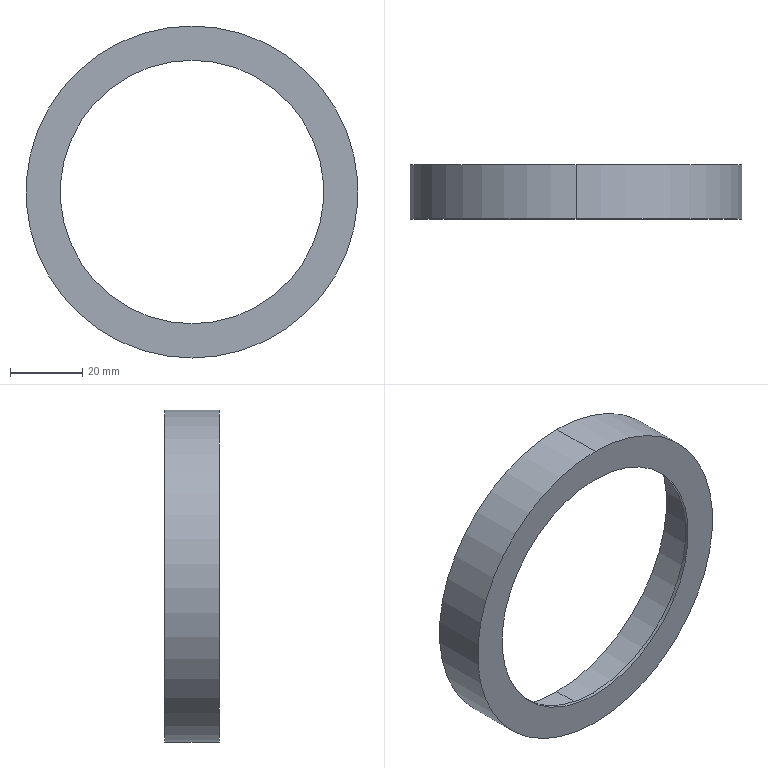Part | SolidWorks | features Revolution 1 | 1 solid | 9 faces | box 92 x 15 x 92 mm | volume 14205 mm3 | cylinder 6 | plane 3 | commonest cylinder face diameters 73 x2 86 x2 92 x2
STEP:
#1=CARTESIAN_POINT('',(0.,15.,43.));
#2=VERTEX_POINT('',#1);
#3=CARTESIAN_POINT('',(0.,15.,-43.));
#4=VERTEX_POINT('',#3);
#5=CARTESIAN_POINT('',(0.,15.,0.));
#6=DIRECTION('',(0.,-1.,0.));
#7=DIRECTION('',(0.,0.,-1.));
#8=AXIS2_PLACEMENT_3D('',#5,#6,#7);
#9=CIRCLE('',#8,43.);
#10=EDGE_CURVE('',#2,#4,#9,.T.);
#11=ORIENTED_EDGE('',*,*,#10,.F.);
#12=CARTESIAN_POINT('',(0.,1.,43.));
#13=VERTEX_POINT('',#12);
#14=CARTESIAN_POINT('',(0.,0.,43.));
#15=DIRECTION('',(0.,-1.,0.));
#16=VECTOR('',#15,1000.);
#17=LINE('',#14,#16);
#18=EDGE_CURVE('',#2,#13,#17,.T.);
#19=ORIENTED_EDGE('',*,*,#18,.T.);
#20=CARTESIAN_POINT('',(0.,1.,-43.));
#21=VERTEX_POINT('',#20);
#22=CARTESIAN_POINT('',(0.,1.,0.));
#23=DIRECTION('',(0.,-1.,0.));
#24=DIRECTION('',(0.,0.,-1.));
#25=AXIS2_PLACEMENT_3D('',#22,#23,#24);
#26=CIRCLE('',#25,43.);
#27=EDGE_CURVE('',#13,#21,#26,.T.);
#28=ORIENTED_EDGE('',*,*,#27,.T.);
#29=CARTESIAN_POINT('',(0.,0.,-43.));
#30=DIRECTION('',(0.,-1.,0.));
#31=VECTOR('',#30,1000.);
#32=LINE('',#29,#31);
#33=EDGE_CURVE('',#4,#21,#32,.T.);
#34=ORIENTED_EDGE('',*,*,#33,.F.);
#35=EDGE_LOOP('',(#11,#19,#28,#34));
#36=FACE_OUTER_BOUND('',#35,.T.);
#37=CARTESIAN_POINT('',(0.,0.,0.));
#38=DIRECTION('',(0.,-1.,0.));
#39=DIRECTION('',(0.,0.,-1.));
#40=AXIS2_PLACEMENT_3D('',#37,#38,#39);
#41=CYLINDRICAL_SURFACE('',#40,43.);
#42=ADVANCED_FACE('',(#36),#41,.F.);
#43=CARTESIAN_POINT('',(0.,1.,36.5));
#44=VERTEX_POINT('',#43);
#45=CARTESIAN_POINT('',(0.,1.,-36.5));
#46=VERTEX_POINT('',#45);
#47=CARTESIAN_POINT('',(0.,1.,0.));
#48=DIRECTION('',(0.,-1.,0.));
#49=DIRECTION('',(0.,0.,-1.));
#50=AXIS2_PLACEMENT_3D('',#47,#48,#49);
#51=CIRCLE('',#50,36.5);
#52=EDGE_CURVE('',#44,#46,#51,.T.);
#53=ORIENTED_EDGE('',*,*,#52,.F.);
#54=CARTESIAN_POINT('',(0.,0.,36.5));
#55=VERTEX_POINT('',#54);
#56=CARTESIAN_POINT('',(0.,0.,36.5));
#57=DIRECTION('',(0.,-1.,0.));
#58=VECTOR('',#57,1000.);
#59=LINE('',#56,#58);
#60=EDGE_CURVE('',#44,#55,#59,.T.);
#61=ORIENTED_EDGE('',*,*,#60,.T.);
#62=CARTESIAN_POINT('',(0.,0.,-36.5));
#63=VERTEX_POINT('',#62);
#64=CARTESIAN_POINT('',(0.,0.,0.));
#65=DIRECTION('',(0.,-1.,0.));
#66=DIRECTION('',(0.,0.,-1.));
#67=AXIS2_PLACEMENT_3D('',#64,#65,#66);
#68=CIRCLE('',#67,36.5);
#69=EDGE_CURVE('',#55,#63,#68,.T.);
#70=ORIENTED_EDGE('',*,*,#69,.T.);
#71=CARTESIAN_POINT('',(0.,0.,-36.5));
#72=DIRECTION('',(0.,-1.,0.));
#73=VECTOR('',#72,1000.);
#74=LINE('',#71,#73);
#75=EDGE_CURVE('',#46,#63,#74,.T.);
#76=ORIENTED_EDGE('',*,*,#75,.F.);
#77=EDGE_LOOP('',(#53,#61,#70,#76));
#78=FACE_OUTER_BOUND('',#77,.T.);
#79=CARTESIAN_POINT('',(0.,0.,0.));
#80=DIRECTION('',(0.,-1.,0.));
#81=DIRECTION('',(0.,0.,-1.));
#82=AXIS2_PLACEMENT_3D('',#79,#80,#81);
#83=CYLINDRICAL_SURFACE('',#82,36.5);
#84=ADVANCED_FACE('',(#78),#83,.F.);
#85=CARTESIAN_POINT('',(0.,15.,-46.));
#86=VERTEX_POINT('',#85);
#87=CARTESIAN_POINT('',(0.,15.,46.));
#88=VERTEX_POINT('',#87);
#89=CARTESIAN_POINT('',(0.,15.,0.));
#90=DIRECTION('',(0.,-1.,0.));
#91=DIRECTION('',(0.,0.,-1.));
#92=AXIS2_PLACEMENT_3D('',#89,#90,#91);
#93=CIRCLE('',#92,46.);
#94=EDGE_CURVE('',#86,#88,#93,.T.);
#95=ORIENTED_EDGE('',*,*,#94,.T.);
#96=CARTESIAN_POINT('',(0.,0.,46.));
#97=VERTEX_POINT('',#96);
#98=CARTESIAN_POINT('',(0.,0.,46.));
#99=DIRECTION('',(0.,-1.,0.));
#100=VECTOR('',#99,1000.);
#101=LINE('',#98,#100);
#102=EDGE_CURVE('',#88,#97,#101,.T.);
#103=ORIENTED_EDGE('',*,*,#102,.T.);
#104=CARTESIAN_POINT('',(0.,0.,-46.));
#105=VERTEX_POINT('',#104);
#106=CARTESIAN_POINT('',(0.,0.,0.));
#107=DIRECTION('',(0.,-1.,0.));
#108=DIRECTION('',(0.,0.,-1.));
#109=AXIS2_PLACEMENT_3D('',#106,#107,#108);
#110=CIRCLE('',#109,46.);
#111=EDGE_CURVE('',#105,#97,#110,.T.);
#112=ORIENTED_EDGE('',*,*,#111,.F.);
#113=CARTESIAN_POINT('',(0.,0.,-46.));
#114=DIRECTION('',(0.,-1.,0.));
#115=VECTOR('',#114,1000.);
#116=LINE('',#113,#115);
#117=EDGE_CURVE('',#86,#105,#116,.T.);
#118=ORIENTED_EDGE('',*,*,#117,.F.);
#119=EDGE_LOOP('',(#95,#103,#112,#118));
#120=FACE_OUTER_BOUND('',#119,.T.);
#121=CARTESIAN_POINT('',(0.,0.,0.));
#122=DIRECTION('',(0.,-1.,0.));
#123=DIRECTION('',(0.,0.,-1.));
#124=AXIS2_PLACEMENT_3D('',#121,#122,#123);
#125=CYLINDRICAL_SURFACE('',#124,46.);
#126=ADVANCED_FACE('',(#120),#125,.T.);
#127=ORIENTED_EDGE('',*,*,#94,.F.);
#128=CARTESIAN_POINT('',(0.,15.,0.));
#129=DIRECTION('',(0.,-1.,0.));
#130=DIRECTION('',(0.,0.,-1.));
#131=AXIS2_PLACEMENT_3D('',#128,#129,#130);
#132=CIRCLE('',#131,46.);
#133=EDGE_CURVE('',#88,#86,#132,.T.);
#134=ORIENTED_EDGE('',*,*,#133,.F.);
#135=EDGE_LOOP('',(#127,#134));
#136=FACE_OUTER_BOUND('',#135,.T.);
#137=CARTESIAN_POINT('',(0.,15.,0.));
#138=DIRECTION('',(0.,-1.,0.));
#139=DIRECTION('',(0.,0.,-1.));
#140=AXIS2_PLACEMENT_3D('',#137,#138,#139);
#141=CIRCLE('',#140,43.);
#142=EDGE_CURVE('',#4,#2,#141,.T.);
#143=ORIENTED_EDGE('',*,*,#142,.T.);
#144=ORIENTED_EDGE('',*,*,#10,.T.);
#145=EDGE_LOOP('',(#143,#144));
#146=FACE_BOUND('',#145,.T.);
#147=CARTESIAN_POINT('',(-43.,15.,0.));
#148=DIRECTION('',(0.,-1.,0.));
#149=DIRECTION('',(0.,0.,-1.));
#150=AXIS2_PLACEMENT_3D('',#147,#148,#149);
#151=PLANE('',#150);
#152=ADVANCED_FACE('',(#136,#146),#151,.F.);
#153=ORIENTED_EDGE('',*,*,#102,.F.);
#154=ORIENTED_EDGE('',*,*,#133,.T.);
#155=ORIENTED_EDGE('',*,*,#117,.T.);
#156=CARTESIAN_POINT('',(0.,0.,0.));
#157=DIRECTION('',(0.,-1.,0.));
#158=DIRECTION('',(0.,0.,-1.));
#159=AXIS2_PLACEMENT_3D('',#156,#157,#158);
#160=CIRCLE('',#159,46.);
#161=EDGE_CURVE('',#97,#105,#160,.T.);
#162=ORIENTED_EDGE('',*,*,#161,.F.);
#163=EDGE_LOOP('',(#153,#154,#155,#162));
#164=FACE_OUTER_BOUND('',#163,.T.);
#165=CARTESIAN_POINT('',(0.,0.,0.));
#166=DIRECTION('',(0.,-1.,0.));
#167=DIRECTION('',(0.,0.,-1.));
#168=AXIS2_PLACEMENT_3D('',#165,#166,#167);
#169=CYLINDRICAL_SURFACE('',#168,46.);
#170=ADVANCED_FACE('',(#164),#169,.T.);
#171=CARTESIAN_POINT('',(0.,0.,0.));
#172=DIRECTION('',(0.,-1.,0.));
#173=DIRECTION('',(0.,0.,-1.));
#174=AXIS2_PLACEMENT_3D('',#171,#172,#173);
#175=CIRCLE('',#174,36.5);
#176=EDGE_CURVE('',#63,#55,#175,.T.);
#177=ORIENTED_EDGE('',*,*,#176,.F.);
#178=ORIENTED_EDGE('',*,*,#69,.F.);
#179=EDGE_LOOP('',(#177,#178));
#180=FACE_BOUND('',#179,.T.);
#181=ORIENTED_EDGE('',*,*,#111,.T.);
#182=ORIENTED_EDGE('',*,*,#161,.T.);
#183=EDGE_LOOP('',(#181,#182));
#184=FACE_OUTER_BOUND('',#183,.T.);
#185=CARTESIAN_POINT('',(-46.,0.,0.));
#186=DIRECTION('',(0.,1.,0.));
#187=DIRECTION('',(0.,0.,1.));
#188=AXIS2_PLACEMENT_3D('',#185,#186,#187);
#189=PLANE('',#188);
#190=ADVANCED_FACE('',(#180,#184),#189,.F.);
#191=ORIENTED_EDGE('',*,*,#60,.F.);
#192=CARTESIAN_POINT('',(0.,1.,0.));
#193=DIRECTION('',(0.,-1.,0.));
#194=DIRECTION('',(0.,0.,-1.));
#195=AXIS2_PLACEMENT_3D('',#192,#193,#194);
#196=CIRCLE('',#195,36.5);
#197=EDGE_CURVE('',#46,#44,#196,.T.);
#198=ORIENTED_EDGE('',*,*,#197,.F.);
#199=ORIENTED_EDGE('',*,*,#75,.T.);
#200=ORIENTED_EDGE('',*,*,#176,.T.);
#201=EDGE_LOOP('',(#191,#198,#199,#200));
#202=FACE_OUTER_BOUND('',#201,.T.);
#203=CARTESIAN_POINT('',(0.,0.,0.));
#204=DIRECTION('',(0.,-1.,0.));
#205=DIRECTION('',(0.,0.,-1.));
#206=AXIS2_PLACEMENT_3D('',#203,#204,#205);
#207=CYLINDRICAL_SURFACE('',#206,36.5);
#208=ADVANCED_FACE('',(#202),#207,.F.);
#209=CARTESIAN_POINT('',(0.,1.,0.));
#210=DIRECTION('',(0.,-1.,0.));
#211=DIRECTION('',(0.,0.,-1.));
#212=AXIS2_PLACEMENT_3D('',#209,#210,#211);
#213=CIRCLE('',#212,43.);
#214=EDGE_CURVE('',#21,#13,#213,.T.);
#215=ORIENTED_EDGE('',*,*,#214,.F.);
#216=ORIENTED_EDGE('',*,*,#27,.F.);
#217=EDGE_LOOP('',(#215,#216));
#218=FACE_OUTER_BOUND('',#217,.T.);
#219=ORIENTED_EDGE('',*,*,#197,.T.);
#220=ORIENTED_EDGE('',*,*,#52,.T.);
#221=EDGE_LOOP('',(#219,#220));
#222=FACE_BOUND('',#221,.T.);
#223=CARTESIAN_POINT('',(-36.5,1.,0.));
#224=DIRECTION('',(0.,-1.,0.));
#225=DIRECTION('',(0.,0.,-1.));
#226=AXIS2_PLACEMENT_3D('',#223,#224,#225);
#227=PLANE('',#226);
#228=ADVANCED_FACE('',(#218,#222),#227,.F.);
#229=ORIENTED_EDGE('',*,*,#18,.F.);
#230=ORIENTED_EDGE('',*,*,#142,.F.);
#231=ORIENTED_EDGE('',*,*,#33,.T.);
#232=ORIENTED_EDGE('',*,*,#214,.T.);
#233=EDGE_LOOP('',(#229,#230,#231,#232));
#234=FACE_OUTER_BOUND('',#233,.T.);
#235=CARTESIAN_POINT('',(0.,0.,0.));
#236=DIRECTION('',(0.,-1.,0.));
#237=DIRECTION('',(0.,0.,-1.));
#238=AXIS2_PLACEMENT_3D('',#235,#236,#237);
#239=CYLINDRICAL_SURFACE('',#238,43.);
#240=ADVANCED_FACE('',(#234),#239,.F.);
#241=CLOSED_SHELL('',(#42,#84,#126,#152,#170,#190,#208,#228,#240));
#242=MANIFOLD_SOLID_BREP('',#241);
#243=CARTESIAN_POINT('',(0.,0.,0.));
#244=DIRECTION('',(0.,0.,1.));
#245=DIRECTION('',(1.,0.,0.));
#246=AXIS2_PLACEMENT_3D('',#243,#244,#245);
#247=(LENGTH_UNIT()NAMED_UNIT(*)SI_UNIT(.MILLI.,.METRE.));
#248=UNCERTAINTY_MEASURE_WITH_UNIT(LENGTH_MEASURE(0.00001),#247,'','');
#249=(NAMED_UNIT(*)PLANE_ANGLE_UNIT()SI_UNIT($,.RADIAN.));
#250=(NAMED_UNIT(*)SI_UNIT($,.STERADIAN.)SOLID_ANGLE_UNIT());
#251=(GEOMETRIC_REPRESENTATION_CONTEXT(3)GLOBAL_UNCERTAINTY_ASSIGNED_CONTEXT((#248))GLOBAL_UNIT_ASSIGNED_CONTEXT((#247,#249,#250))REPRESENTATION_CONTEXT('',''));
#252=ADVANCED_BREP_SHAPE_REPRESENTATION('',(#242,#246),#251);